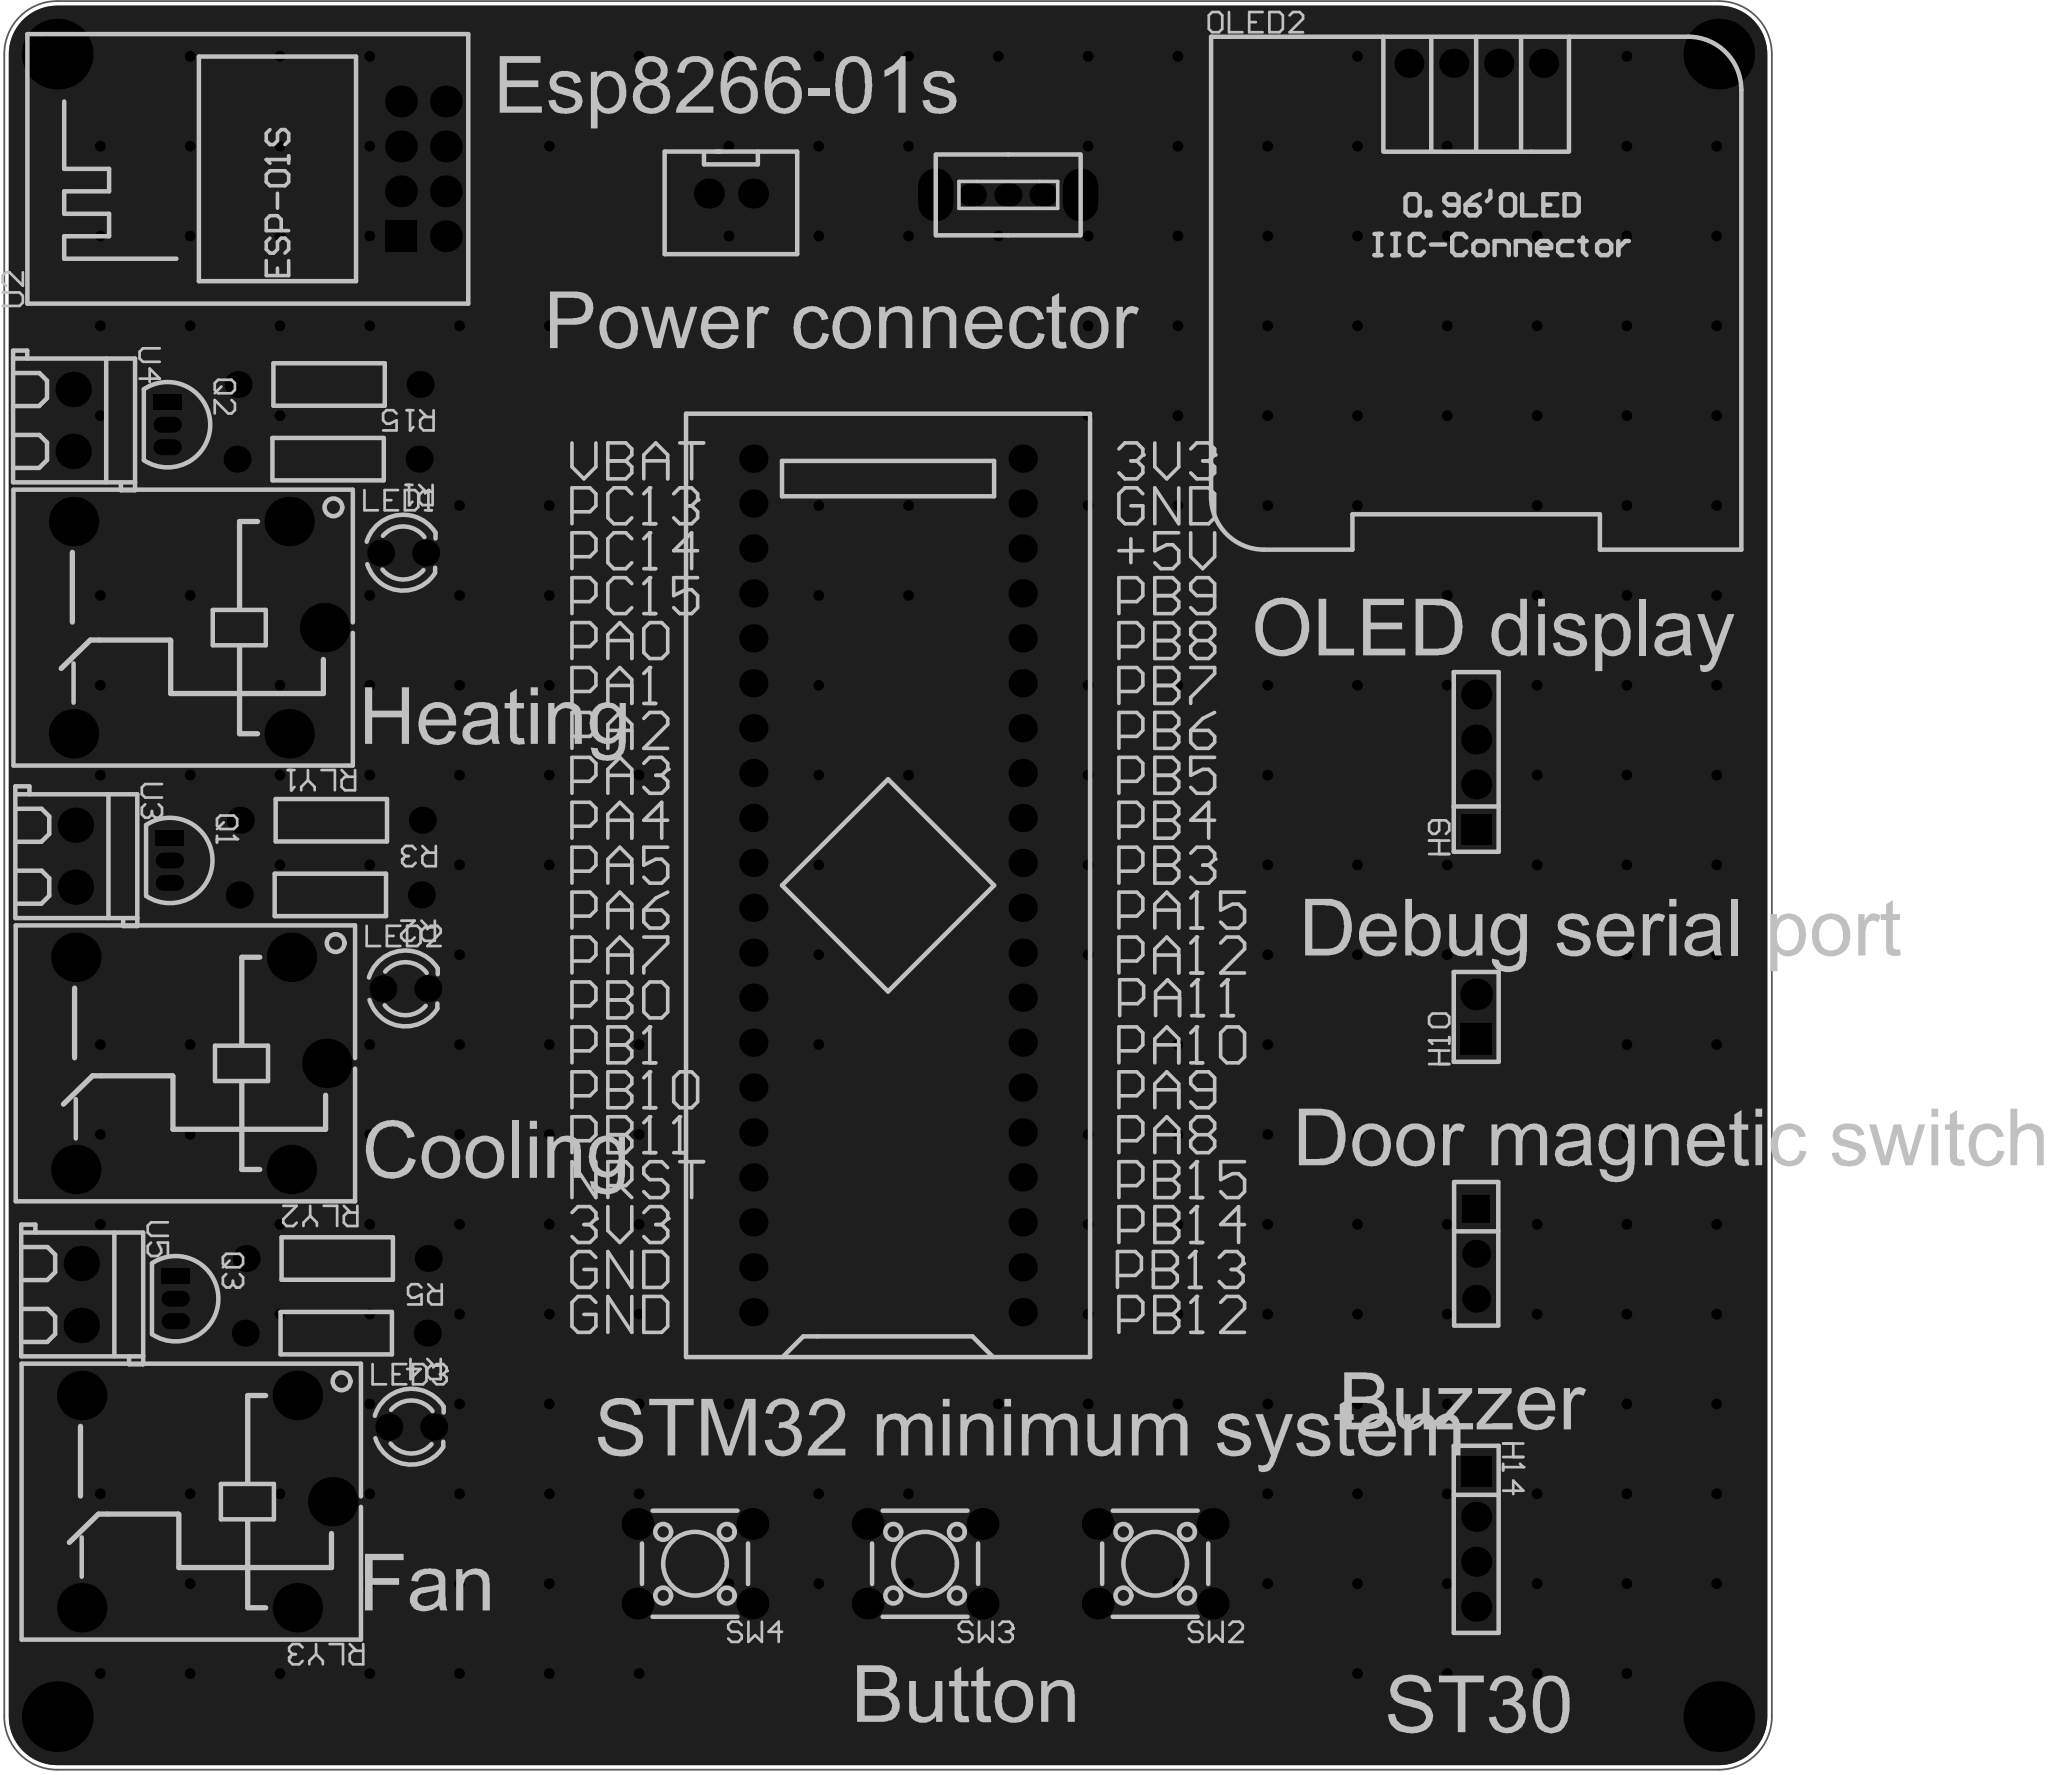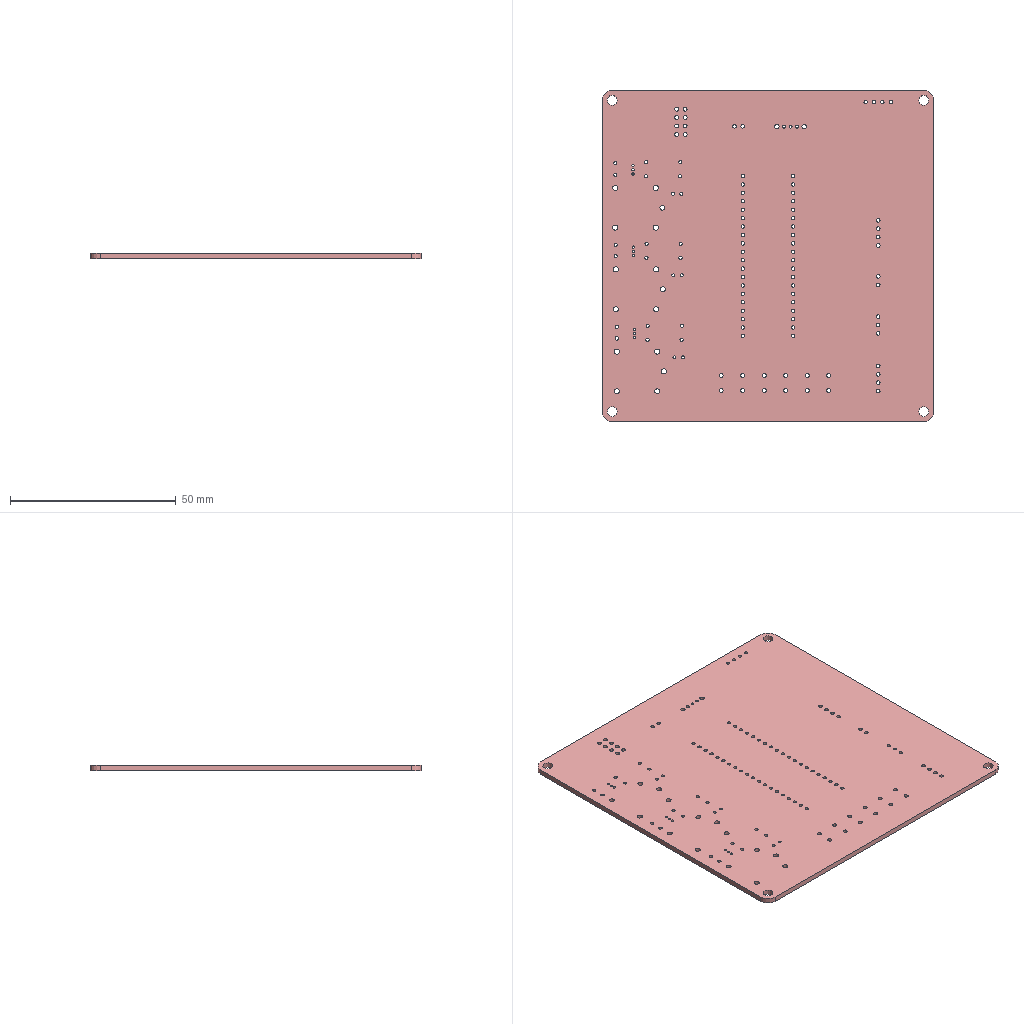Circuit board layout | Altium Designer | box 100 x 100 x 1.6 mm
Layer stack:
# Altium Designer layer stack of  (unit mm; dielectric type: 0 none, 1 core, 2 prepreg, 3 surface material)
index,name,kind,layer,copper_thickness_mm,dielectric_type,dielectric_thickness_mm,dielectric_material,dielectric_constant
0,Top Paste Mask Layer,other,,,,,,
1,Top Silkscreen Layer,other,,,,,,
2,Top Solder Mask Layer,dielectric,,,3,0.01,,3.3
3,Top Layer,copper,Top Layer,0.035,,,,
4,Dielectric1,dielectric,,,3,1.51,FR4,4.5
5,Bottom Layer,copper,Bottom Layer,0.035,,,,
6,Bottom Solder Mask Layer,dielectric,,,3,0.01,,3.3
7,Bottom Silkscreen Layer,other,,,,,,
8,Bottom Paste Mask Layer,other,,,,,,
# drill layer pairs: low layer,high layer
drill_pair,Top Layer,Bottom Layer
Part placement:
Designator,Comment,Layer,Footprint,Center-X(mm),Center-Y(mm),Rotation
U1,STM32F103C8T6-Card,TopLayer,CONN-TH_L53.3-W22.9_STM32F103C8T6-CARD,141.351,130.937,90
SW2,,TopLayer,SW-TH_4P-L6.0-W6.0-P4.50-LS6.5,156.464,92.583,180
SW3,,TopLayer,SW-TH_4P-L6.0-W6.0-P4.50-LS6.5,143.446,92.583,180
SW4,,TopLayer,SW-TH_4P-L6.0-W6.0-P4.50-LS6.5,130.429,92.583,180
CN4,XH2.54*2P_THT,TopLayer,CONN-TH_2P-P2.50-XH2.54-2P,132.461,170.053,0
SW5,,TopLayer,拨动开关,148.148,169.978,180
H1,,TopLayer,HDR-TH_3P-P2.54-V-F,174.625,110.106,270
OLED2,,TopLayer,0.96OLED_4P,174.625,177.419,0
H9,,TopLayer,HDR-TH_4P-P2.54-V-M,174.625,137.916,90
H10,,TopLayer,HDR-TH_2P-P2.54-V-M-1,174.625,123.501,90
H14,,TopLayer,HDR-TH_4P-P2.54-V-F,174.625,93.961,270
LED1,,TopLayer,LED_TH-3mm,113.919,149.733,0
LED2,,TopLayer,LED_TH-3mm,114.046,125.095,0
LED3,,TopLayer,LED_TH-3mm,114.38,100.315,0
Q1,,TopLayer,S8050_TO_92,100.72,132.346,270
Q2,,TopLayer,S8050_TO_92,100.593,156.984,270
Q3,,TopLayer,S8050_TO_92,101.054,107.566,270
R1,1kΩ,TopLayer,Res_1/4W,109.672,155.037,180
R2,1kΩ,TopLayer,Res_1/4W,109.799,130.399,180
R3,1kΩ,TopLayer,Res_1/4W,109.855,134.62,180
R4,1kΩ,TopLayer,Res_1/4W,110.133,105.619,180
R5,1kΩ,TopLayer,Res_1/4W,110.189,109.84,180
R15,1kΩ,TopLayer,Res_1/4W,109.728,159.258,180
RLY1,SRD-05VDC-SL-C,TopLayer,RELAY-TH_SRD-XXVDC-XL-C,102.371,145.512,180
RLY2,SRD-05VDC-SL-C,TopLayer,RELAY-TH_SRD-XXVDC-XL-C,102.498,120.874,180
RLY3,SRD-05VDC-SL-C,TopLayer,RELAY-TH_SRD-XXVDC-XL-C,102.832,96.094,180
U2,ESP-01S,TopLayer,WIFIM-TH_ESP-01S,115.062,171.45,90
U3,KF350-3.5-2P,TopLayer,CONN-TH_P3.50_KF350-3.5-2P,95.377,132.588,270
U4,KF350-3.5-2P,TopLayer,CONN-TH_P3.50_KF350-3.5-2P,95.25,157.226,270
U5,KF350-3.5-2P,TopLayer,CONN-TH_P3.50_KF350-3.5-2P,95.711,107.808,270
Pad and via stacks:
# Altium Designer via and pad stacks of  (unit mm). Each distinct definition once, with the count of objects using it.
# via: kind,start_layer,end_layer,hole_mm,diameter_mm,mode(0 simple;1 top-mid-bottom;2 full stack),diameter_per_layer,count,example_net
# pad: kind,layer,hole_mm,hole_type(0 round;1 square;2 slot),plating,top_size,top_shape(1 round;2 rect;3 octagon;9 rounded rect),mid_size,bottom_size,mode,footprint,size_per_layer,count,example
pad,Multi-Layer,3,0,plated,4x4,1,4x4,4x4,0,,,4,1
pad,Multi-Layer,1,0,plated,1.6x1.6,1,1.6x1.6,1.6x1.6,0,CONN-TH_L53.3-W22.9_STM32F103C8T6-CARD,,40,U1.1
pad,Multi-Layer,1.2,0,plated,1.8x1.8,1,1.8x1.8,1.8x1.8,0,SW-TH_4P-L6.0-W6.0-P4.50-LS6.5,,12,SW2.1
pad,Multi-Layer,1.05,0,plated,1.7x1.7,1,1.7x1.7,1.7x1.7,0,CONN-TH_2P-P2.50-XH2.54-2P,,2,CN4.2
pad,Multi-Layer,0.8992,0,plated,1.6x1.3,1,1.6x1.3,1.6x1.3,0,\u00B2\u00A6\u00B6\u00AF\u00BF\u00AA\u00B9\u00D8,,3,SW5.1
pad,Multi-Layer,1.3,0,plated,3x1.999,1,3x1.999,3x1.999,0,\u00B2\u00A6\u00B6\u00AF\u00BF\u00AA\u00B9\u00D8,,2,SW5.4
pad,Multi-Layer,1.02,0,plated,1.575x1.575,1,1.575x1.575,1.575x1.575,0,HDR-TH_3P-P2.54-V-F,,2,H1.3
pad,Multi-Layer,1.02,0,plated,1.575x1.575,2,1.575x1.575,1.575x1.575,0,HDR-TH_3P-P2.54-V-F,,1,H1.1
pad,Multi-Layer,1,0,plated,1.65x1.65,1,1.65x1.65,1.65x1.65,0,0.96OLED_4P,,4,OLED2.4
pad,Multi-Layer,1.1,0,plated,1.7x1.7,2,1.7x1.7,1.7x1.7,0,HDR-TH_4P-P2.54-V-M,,1,H9.1
pad,Multi-Layer,1.1,0,plated,1.7x1.7,1,1.7x1.7,1.7x1.7,0,HDR-TH_4P-P2.54-V-M,,3,H9.2
pad,Multi-Layer,1.1,0,plated,1.8x1.8,1,1.8x1.8,1.8x1.8,0,HDR-TH_2P-P2.54-V-M-1,,1,H10.2
pad,Multi-Layer,1.1,0,plated,1.8x1.8,2,1.8x1.8,1.8x1.8,0,HDR-TH_2P-P2.54-V-M-1,,1,H10.1
pad,Multi-Layer,1.1,0,plated,1.7x1.7,2,1.7x1.7,1.7x1.7,0,HDR-TH_4P-P2.54-V-F,,1,H14.1
pad,Multi-Layer,1.1,0,plated,1.7x1.7,1,1.7x1.7,1.7x1.7,0,HDR-TH_4P-P2.54-V-F,,3,H14.2
pad,Multi-Layer,0.9144,0,plated,1.524x1.524,1,1.524x1.524,1.524x1.524,0,LED_TH-3mm,,6,LED1.1
pad,Multi-Layer,0.701,0,plated,0.8992x1.6,2,0.8992x1.6,0.8992x1.6,0,S8050_TO_92,,3,Q1.1
pad,Multi-Layer,0.701,0,plated,0.8992x1.6,1,0.8992x1.6,0.8992x1.6,0,S8050_TO_92,,6,Q1.2
pad,Multi-Layer,1,0,plated,1.524x1.524,1,1.524x1.524,1.524x1.524,0,Res_1/4W,,12,R1.1
pad,Multi-Layer,1.524,0,plated,2.794x2.794,1,2.794x2.794,2.794x2.794,0,RELAY-TH_SRD-XXVDC-XL-C,,15,RLY1.2
pad,Multi-Layer,1.2,0,plated,1.8x1.8,2,1.8x1.8,1.8x1.8,0,WIFIM-TH_ESP-01S,,1,U2.1
pad,Multi-Layer,1.2,0,plated,1.8x1.8,1,1.8x1.8,1.8x1.8,0,WIFIM-TH_ESP-01S,,7,U2.2
pad,Multi-Layer,1,0,plated,2x2,1,2x2,2x2,0,CONN-TH_P3.50_KF350-3.5-2P,,6,U3.1
via,Top Layer,Bottom Layer,0.3048,0.61,0,,242,GND
Copper pours:
name,layer,net,type(0 solid;1 hatched;2 none)
Bottom Layer-GND,Bottom Layer,GND,0
Top Layer-GND,Top Layer,GND,0
Design rules, without the lines most boards share:
# Altium Designer design rules of  (exported by Altium Designer, unit mm)
# columns: name | kind | enabled | priority | scope1 | scope2 | descriptor | typed fields (field=value)
Copper_copperRegion_copperThickness1oz | 0 | disabled | 4 | All | All | Clearance Constraint (Gap=5.984mil) (Disabled)(All),(All) | gap=0.152
Copper_copperRegion_copperThickness1oz_1 | 63 | disabled | 4 | All | All | Board Clearance Constraint (Gap=0mil) (Disabled)(All) |
Copper_copperRegion_Copper_copperRegion | 0 | disabled | 5 | All | All | Clearance Constraint (Gap=5.984mil) (Disabled)(All),(All) | gap=0.152
Copper_copperRegion_Copper_copperRegion_1 | 63 | disabled | 5 | All | All | Board Clearance Constraint (Gap=0mil) (Disabled)(All) |
copperThickness1oz | 0 | enabled | 6 | All | All | Clearance Constraint (Gap=5.984mil) (All),(All) | gap=0.152
copperThickness1oz_1 | 63 | enabled | 6 | All | All | Board Clearance Constraint (Gap=0mil) (All) |
copperRegion_copperThickness1oz | 20 | disabled | 1 | All | All | Polygon Connect Rule(Relief Connect )(Conductor Width=10mil) (Relief Angle=90 Angle) (Entries=4) (Air Gap Width=10mil) (Disabled)(All),(All) | connect_style(0=relief,1=direct,2=none)=0 relief_conductor_width=0.254 relief_entries=4
copperRegion_Copper_copperRegion | 20 | disabled | 2 | All | All | Polygon Connect Rule(Relief Connect )(Conductor Width=10mil) (Relief Angle=90 Angle) (Entries=4) (Air Gap Width=10mil) (Disabled)(All),(All) | connect_style(0=relief,1=direct,2=none)=0 relief_conductor_width=0.254 relief_entries=4
copperRegion | 20 | enabled | 3 | All | All | Polygon Connect Rule(Relief Connect )(Conductor Width=10mil) (Relief Angle=90 Angle) (Entries=4) (Air Gap Width=10mil) (All),(All) | connect_style(0=relief,1=direct,2=none)=0 relief_conductor_width=0.254 relief_entries=4